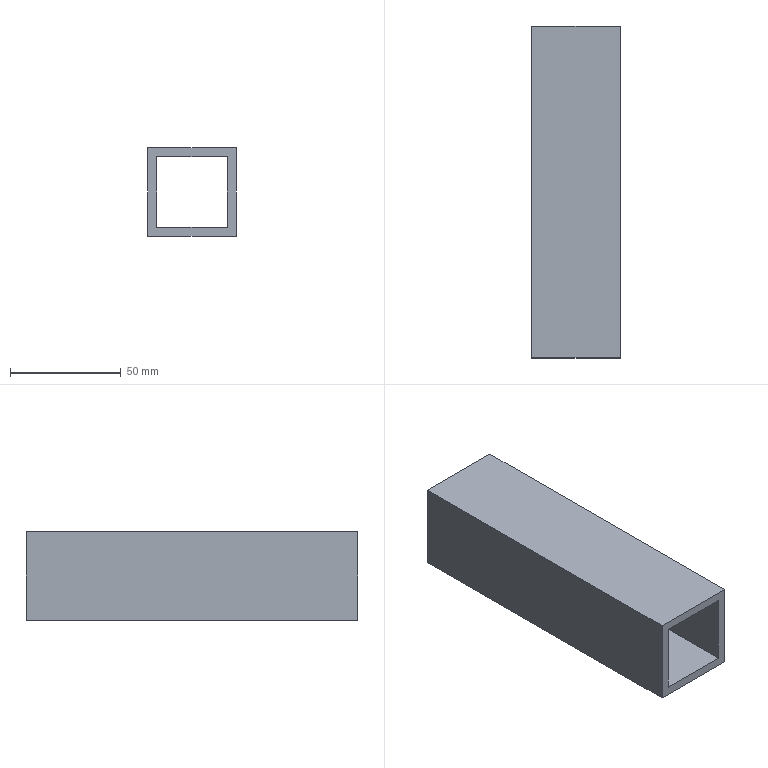Part | NX | features solid 2 | 1 solid | 10 faces | box 40 x 150 x 40 mm | volume 86400 mm3 | plane 10
STEP:
#1=CARTESIAN_POINT('',(655.,-20.,-45.));
#2=VERTEX_POINT('',#1);
#3=CARTESIAN_POINT('',(655.,130.,-45.));
#4=VERTEX_POINT('',#3);
#5=CARTESIAN_POINT('',(655.,1714.393,-45.));
#6=DIRECTION('',(0.,1.,0.));
#7=VECTOR('',#6,1000.);
#8=LINE('',#5,#7);
#9=EDGE_CURVE('',#2,#4,#8,.T.);
#10=ORIENTED_EDGE('',*,*,#9,.T.);
#11=CARTESIAN_POINT('',(655.,130.,-85.));
#12=VERTEX_POINT('',#11);
#13=CARTESIAN_POINT('',(655.,130.,-70.));
#14=DIRECTION('',(0.,0.,1.));
#15=VECTOR('',#14,1000.);
#16=LINE('',#13,#15);
#17=EDGE_CURVE('',#12,#4,#16,.T.);
#18=ORIENTED_EDGE('',*,*,#17,.F.);
#19=CARTESIAN_POINT('',(655.,-20.,-85.));
#20=VERTEX_POINT('',#19);
#21=CARTESIAN_POINT('',(655.,1629.393,-85.));
#22=DIRECTION('',(0.,1.,0.));
#23=VECTOR('',#22,1000.);
#24=LINE('',#21,#23);
#25=EDGE_CURVE('',#20,#12,#24,.T.);
#26=ORIENTED_EDGE('',*,*,#25,.F.);
#27=CARTESIAN_POINT('',(655.,-20.,-70.));
#28=DIRECTION('',(0.,0.,-1.));
#29=VECTOR('',#28,1000.);
#30=LINE('',#27,#29);
#31=EDGE_CURVE('',#2,#20,#30,.T.);
#32=ORIENTED_EDGE('',*,*,#31,.F.);
#33=EDGE_LOOP('',(#10,#18,#26,#32));
#34=FACE_BOUND('',#33,.T.);
#35=CARTESIAN_POINT('',(655.,1629.393,-70.));
#36=DIRECTION('',(1.,0.,0.));
#37=DIRECTION('',(0.,0.,1.));
#38=AXIS2_PLACEMENT_3D('',#35,#36,#37);
#39=PLANE('',#38);
#40=ADVANCED_FACE('',(#34),#39,.F.);
#41=ORIENTED_EDGE('',*,*,#25,.T.);
#42=CARTESIAN_POINT('',(695.,130.,-85.));
#43=VERTEX_POINT('',#42);
#44=CARTESIAN_POINT('',(75.,130.,-85.));
#45=DIRECTION('',(-1.,0.,0.));
#46=VECTOR('',#45,1000.);
#47=LINE('',#44,#46);
#48=EDGE_CURVE('',#43,#12,#47,.T.);
#49=ORIENTED_EDGE('',*,*,#48,.F.);
#50=CARTESIAN_POINT('',(695.,-20.,-85.));
#51=VERTEX_POINT('',#50);
#52=CARTESIAN_POINT('',(695.,1714.393,-85.));
#53=DIRECTION('',(0.,1.,0.));
#54=VECTOR('',#53,1000.);
#55=LINE('',#52,#54);
#56=EDGE_CURVE('',#51,#43,#55,.T.);
#57=ORIENTED_EDGE('',*,*,#56,.F.);
#58=CARTESIAN_POINT('',(75.,-20.,-85.));
#59=DIRECTION('',(1.,0.,0.));
#60=VECTOR('',#59,1000.);
#61=LINE('',#58,#60);
#62=EDGE_CURVE('',#20,#51,#61,.T.);
#63=ORIENTED_EDGE('',*,*,#62,.F.);
#64=EDGE_LOOP('',(#41,#49,#57,#63));
#65=FACE_BOUND('',#64,.T.);
#66=CARTESIAN_POINT('',(75.,1714.393,-85.));
#67=DIRECTION('',(0.,0.,1.));
#68=DIRECTION('',(-1.,0.,0.));
#69=AXIS2_PLACEMENT_3D('',#66,#67,#68);
#70=PLANE('',#69);
#71=ADVANCED_FACE('',(#65),#70,.F.);
#72=CARTESIAN_POINT('',(695.,130.,-45.));
#73=VERTEX_POINT('',#72);
#74=CARTESIAN_POINT('',(695.,-20.,-45.));
#75=VERTEX_POINT('',#74);
#76=CARTESIAN_POINT('',(695.,1714.393,-45.));
#77=DIRECTION('',(0.,-1.,0.));
#78=VECTOR('',#77,1000.);
#79=LINE('',#76,#78);
#80=EDGE_CURVE('',#73,#75,#79,.T.);
#81=ORIENTED_EDGE('',*,*,#80,.F.);
#82=CARTESIAN_POINT('',(35.,130.,-45.));
#83=DIRECTION('',(1.,0.,0.));
#84=VECTOR('',#83,1000.);
#85=LINE('',#82,#84);
#86=EDGE_CURVE('',#4,#73,#85,.T.);
#87=ORIENTED_EDGE('',*,*,#86,.F.);
#88=ORIENTED_EDGE('',*,*,#9,.F.);
#89=CARTESIAN_POINT('',(35.,-20.,-45.));
#90=DIRECTION('',(-1.,0.,0.));
#91=VECTOR('',#90,1000.);
#92=LINE('',#89,#91);
#93=EDGE_CURVE('',#75,#2,#92,.T.);
#94=ORIENTED_EDGE('',*,*,#93,.F.);
#95=EDGE_LOOP('',(#81,#87,#88,#94));
#96=FACE_BOUND('',#95,.T.);
#97=CARTESIAN_POINT('',(35.,1714.393,-45.));
#98=DIRECTION('',(0.,0.,-1.));
#99=DIRECTION('',(1.,0.,0.));
#100=AXIS2_PLACEMENT_3D('',#97,#98,#99);
#101=PLANE('',#100);
#102=ADVANCED_FACE('',(#96),#101,.F.);
#103=ORIENTED_EDGE('',*,*,#56,.T.);
#104=CARTESIAN_POINT('',(695.,130.,-40.));
#105=DIRECTION('',(0.,0.,-1.));
#106=VECTOR('',#105,1000.);
#107=LINE('',#104,#106);
#108=EDGE_CURVE('',#73,#43,#107,.T.);
#109=ORIENTED_EDGE('',*,*,#108,.F.);
#110=ORIENTED_EDGE('',*,*,#80,.T.);
#111=CARTESIAN_POINT('',(695.,-20.,-40.));
#112=DIRECTION('',(0.,0.,1.));
#113=VECTOR('',#112,1000.);
#114=LINE('',#111,#113);
#115=EDGE_CURVE('',#51,#75,#114,.T.);
#116=ORIENTED_EDGE('',*,*,#115,.F.);
#117=EDGE_LOOP('',(#103,#109,#110,#116));
#118=FACE_BOUND('',#117,.T.);
#119=CARTESIAN_POINT('',(695.,1629.393,-40.));
#120=DIRECTION('',(-1.,0.,0.));
#121=DIRECTION('',(0.,0.,-1.));
#122=AXIS2_PLACEMENT_3D('',#119,#120,#121);
#123=PLANE('',#122);
#124=ADVANCED_FACE('',(#118),#123,.F.);
#125=CARTESIAN_POINT('',(659.,-20.,-49.));
#126=VERTEX_POINT('',#125);
#127=CARTESIAN_POINT('',(659.,-20.,-81.));
#128=VERTEX_POINT('',#127);
#129=CARTESIAN_POINT('',(659.,-20.,-70.));
#130=DIRECTION('',(0.,0.,-1.));
#131=VECTOR('',#130,1000.);
#132=LINE('',#129,#131);
#133=EDGE_CURVE('',#126,#128,#132,.T.);
#134=ORIENTED_EDGE('',*,*,#133,.T.);
#135=CARTESIAN_POINT('',(659.,130.,-81.));
#136=VERTEX_POINT('',#135);
#137=CARTESIAN_POINT('',(659.,1629.393,-81.));
#138=DIRECTION('',(0.,1.,0.));
#139=VECTOR('',#138,1000.);
#140=LINE('',#137,#139);
#141=EDGE_CURVE('',#128,#136,#140,.T.);
#142=ORIENTED_EDGE('',*,*,#141,.T.);
#143=CARTESIAN_POINT('',(659.,130.,-49.));
#144=VERTEX_POINT('',#143);
#145=CARTESIAN_POINT('',(659.,130.,-70.));
#146=DIRECTION('',(0.,0.,1.));
#147=VECTOR('',#146,1000.);
#148=LINE('',#145,#147);
#149=EDGE_CURVE('',#136,#144,#148,.T.);
#150=ORIENTED_EDGE('',*,*,#149,.T.);
#151=CARTESIAN_POINT('',(659.,1714.393,-49.));
#152=DIRECTION('',(0.,1.,0.));
#153=VECTOR('',#152,1000.);
#154=LINE('',#151,#153);
#155=EDGE_CURVE('',#126,#144,#154,.T.);
#156=ORIENTED_EDGE('',*,*,#155,.F.);
#157=EDGE_LOOP('',(#134,#142,#150,#156));
#158=FACE_BOUND('',#157,.T.);
#159=CARTESIAN_POINT('',(659.,1629.393,-70.));
#160=DIRECTION('',(1.,0.,0.));
#161=DIRECTION('',(0.,0.,1.));
#162=AXIS2_PLACEMENT_3D('',#159,#160,#161);
#163=PLANE('',#162);
#164=ADVANCED_FACE('',(#158),#163,.T.);
#165=CARTESIAN_POINT('',(691.,-20.,-81.));
#166=VERTEX_POINT('',#165);
#167=CARTESIAN_POINT('',(75.,-20.,-81.));
#168=DIRECTION('',(1.,0.,0.));
#169=VECTOR('',#168,1000.);
#170=LINE('',#167,#169);
#171=EDGE_CURVE('',#128,#166,#170,.T.);
#172=ORIENTED_EDGE('',*,*,#171,.T.);
#173=CARTESIAN_POINT('',(691.,130.,-81.));
#174=VERTEX_POINT('',#173);
#175=CARTESIAN_POINT('',(691.,1714.393,-81.));
#176=DIRECTION('',(0.,1.,0.));
#177=VECTOR('',#176,1000.);
#178=LINE('',#175,#177);
#179=EDGE_CURVE('',#166,#174,#178,.T.);
#180=ORIENTED_EDGE('',*,*,#179,.T.);
#181=CARTESIAN_POINT('',(75.,130.,-81.));
#182=DIRECTION('',(-1.,0.,0.));
#183=VECTOR('',#182,1000.);
#184=LINE('',#181,#183);
#185=EDGE_CURVE('',#174,#136,#184,.T.);
#186=ORIENTED_EDGE('',*,*,#185,.T.);
#187=ORIENTED_EDGE('',*,*,#141,.F.);
#188=EDGE_LOOP('',(#172,#180,#186,#187));
#189=FACE_BOUND('',#188,.T.);
#190=CARTESIAN_POINT('',(75.,1714.393,-81.));
#191=DIRECTION('',(0.,0.,1.));
#192=DIRECTION('',(-1.,0.,0.));
#193=AXIS2_PLACEMENT_3D('',#190,#191,#192);
#194=PLANE('',#193);
#195=ADVANCED_FACE('',(#189),#194,.T.);
#196=CARTESIAN_POINT('',(691.,-20.,-49.));
#197=VERTEX_POINT('',#196);
#198=CARTESIAN_POINT('',(35.,-20.,-49.));
#199=DIRECTION('',(-1.,0.,0.));
#200=VECTOR('',#199,1000.);
#201=LINE('',#198,#200);
#202=EDGE_CURVE('',#197,#126,#201,.T.);
#203=ORIENTED_EDGE('',*,*,#202,.T.);
#204=ORIENTED_EDGE('',*,*,#155,.T.);
#205=CARTESIAN_POINT('',(691.,130.,-49.));
#206=VERTEX_POINT('',#205);
#207=CARTESIAN_POINT('',(35.,130.,-49.));
#208=DIRECTION('',(1.,0.,0.));
#209=VECTOR('',#208,1000.);
#210=LINE('',#207,#209);
#211=EDGE_CURVE('',#144,#206,#210,.T.);
#212=ORIENTED_EDGE('',*,*,#211,.T.);
#213=CARTESIAN_POINT('',(691.,1714.393,-49.));
#214=DIRECTION('',(0.,-1.,0.));
#215=VECTOR('',#214,1000.);
#216=LINE('',#213,#215);
#217=EDGE_CURVE('',#206,#197,#216,.T.);
#218=ORIENTED_EDGE('',*,*,#217,.T.);
#219=EDGE_LOOP('',(#203,#204,#212,#218));
#220=FACE_BOUND('',#219,.T.);
#221=CARTESIAN_POINT('',(35.,1714.393,-49.));
#222=DIRECTION('',(0.,0.,-1.));
#223=DIRECTION('',(1.,0.,0.));
#224=AXIS2_PLACEMENT_3D('',#221,#222,#223);
#225=PLANE('',#224);
#226=ADVANCED_FACE('',(#220),#225,.T.);
#227=CARTESIAN_POINT('',(691.,-20.,-40.));
#228=DIRECTION('',(0.,0.,1.));
#229=VECTOR('',#228,1000.);
#230=LINE('',#227,#229);
#231=EDGE_CURVE('',#166,#197,#230,.T.);
#232=ORIENTED_EDGE('',*,*,#231,.T.);
#233=ORIENTED_EDGE('',*,*,#217,.F.);
#234=CARTESIAN_POINT('',(691.,130.,-40.));
#235=DIRECTION('',(0.,0.,-1.));
#236=VECTOR('',#235,1000.);
#237=LINE('',#234,#236);
#238=EDGE_CURVE('',#206,#174,#237,.T.);
#239=ORIENTED_EDGE('',*,*,#238,.T.);
#240=ORIENTED_EDGE('',*,*,#179,.F.);
#241=EDGE_LOOP('',(#232,#233,#239,#240));
#242=FACE_BOUND('',#241,.T.);
#243=CARTESIAN_POINT('',(691.,1629.393,-40.));
#244=DIRECTION('',(-1.,0.,0.));
#245=DIRECTION('',(0.,0.,-1.));
#246=AXIS2_PLACEMENT_3D('',#243,#244,#245);
#247=PLANE('',#246);
#248=ADVANCED_FACE('',(#242),#247,.T.);
#249=ORIENTED_EDGE('',*,*,#185,.F.);
#250=ORIENTED_EDGE('',*,*,#238,.F.);
#251=ORIENTED_EDGE('',*,*,#211,.F.);
#252=ORIENTED_EDGE('',*,*,#149,.F.);
#253=EDGE_LOOP('',(#249,#250,#251,#252));
#254=FACE_BOUND('',#253,.T.);
#255=ORIENTED_EDGE('',*,*,#17,.T.);
#256=ORIENTED_EDGE('',*,*,#86,.T.);
#257=ORIENTED_EDGE('',*,*,#108,.T.);
#258=ORIENTED_EDGE('',*,*,#48,.T.);
#259=EDGE_LOOP('',(#255,#256,#257,#258));
#260=FACE_BOUND('',#259,.T.);
#261=CARTESIAN_POINT('',(655.,130.,-45.));
#262=DIRECTION('',(0.,-1.,0.));
#263=DIRECTION('',(0.,0.,-1.));
#264=AXIS2_PLACEMENT_3D('',#261,#262,#263);
#265=PLANE('',#264);
#266=ADVANCED_FACE('',(#254,#260),#265,.F.);
#267=ORIENTED_EDGE('',*,*,#133,.F.);
#268=ORIENTED_EDGE('',*,*,#202,.F.);
#269=ORIENTED_EDGE('',*,*,#231,.F.);
#270=ORIENTED_EDGE('',*,*,#171,.F.);
#271=EDGE_LOOP('',(#267,#268,#269,#270));
#272=FACE_BOUND('',#271,.T.);
#273=ORIENTED_EDGE('',*,*,#93,.T.);
#274=ORIENTED_EDGE('',*,*,#31,.T.);
#275=ORIENTED_EDGE('',*,*,#62,.T.);
#276=ORIENTED_EDGE('',*,*,#115,.T.);
#277=EDGE_LOOP('',(#273,#274,#275,#276));
#278=FACE_BOUND('',#277,.T.);
#279=CARTESIAN_POINT('',(695.,-20.,-45.));
#280=DIRECTION('',(0.,1.,0.));
#281=DIRECTION('',(0.,0.,1.));
#282=AXIS2_PLACEMENT_3D('',#279,#280,#281);
#283=PLANE('',#282);
#284=ADVANCED_FACE('',(#272,#278),#283,.F.);
#285=CLOSED_SHELL('',(#40,#71,#102,#124,#164,#195,#226,#248,#266,#284));
#286=MANIFOLD_SOLID_BREP('',#285);
#287=(LENGTH_UNIT()NAMED_UNIT(*)SI_UNIT(.MILLI.,.METRE.));
#288=UNCERTAINTY_MEASURE_WITH_UNIT(LENGTH_MEASURE(0.00001),#287,'','');
#289=(NAMED_UNIT(*)PLANE_ANGLE_UNIT()SI_UNIT($,.RADIAN.));
#290=(NAMED_UNIT(*)SI_UNIT($,.STERADIAN.)SOLID_ANGLE_UNIT());
#291=(GEOMETRIC_REPRESENTATION_CONTEXT(3)GLOBAL_UNCERTAINTY_ASSIGNED_CONTEXT((#288))GLOBAL_UNIT_ASSIGNED_CONTEXT((#287,#289,#290))REPRESENTATION_CONTEXT('',''));
#292=ADVANCED_BREP_SHAPE_REPRESENTATION('',(#286),#291);